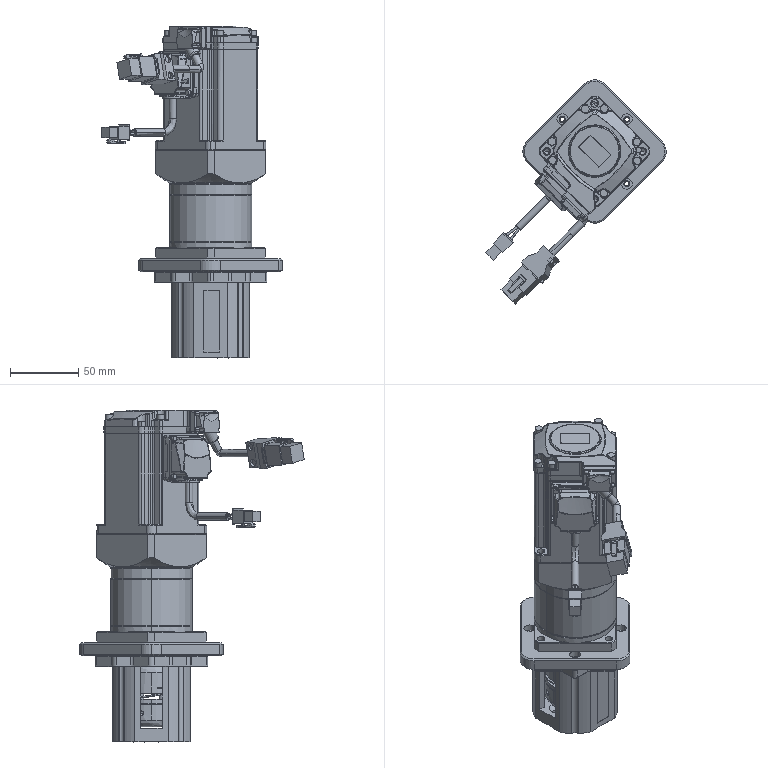Part | STEP file | Copy of 400W gearbox assembly (universal motor base plus Q15)^K50A-1H20-S(formula driven)-L1200 right | 11 solids | 1691 faces | box 131.976 x 164.111 x 242.5 mm | volume 720796 mm3 | cylinder 597 | plane 547 | spline 336 | cone 201 | torus 10 | commonest cylinder face diameters 1 x86 4 x48 0.4 x45 6 x44 5.5 x38 3.5 x28